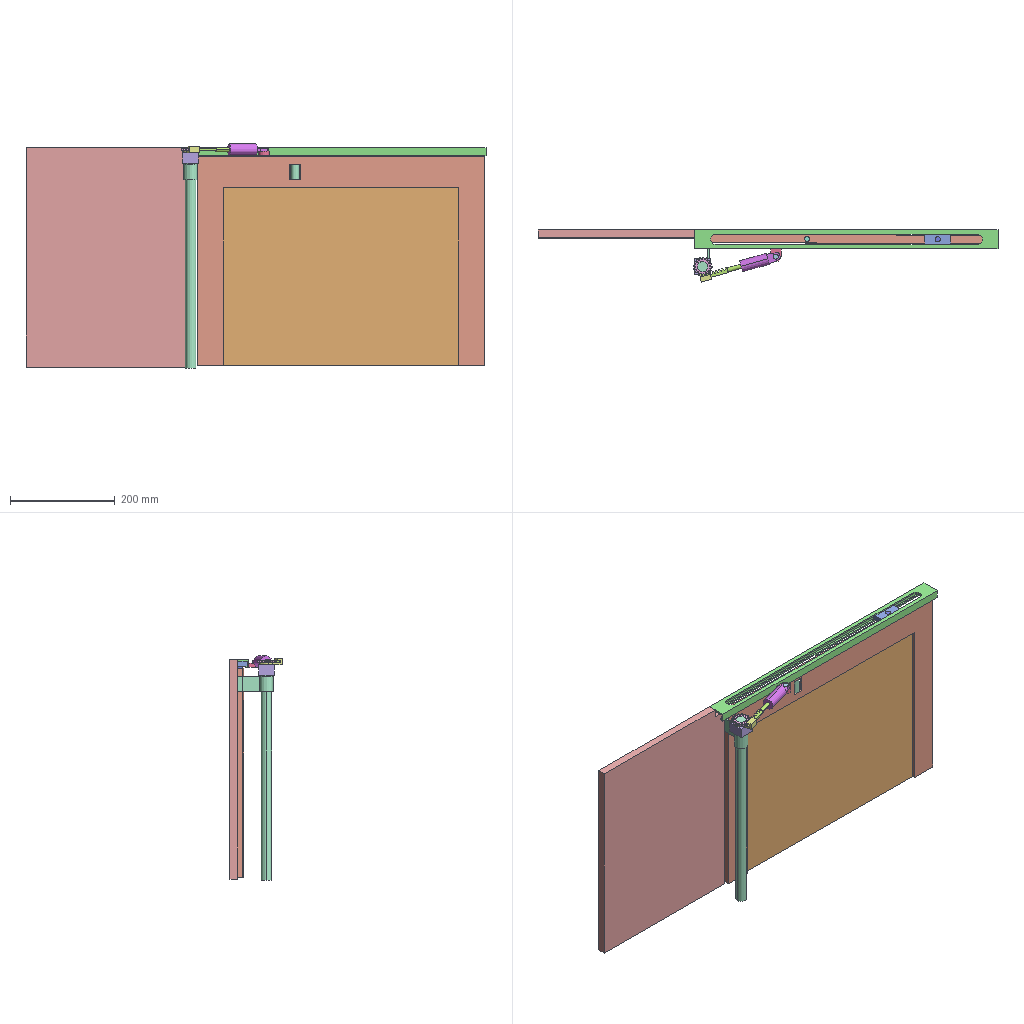Assembly | SolidWorks | 14 different items | 14 placed | box 880 x 100 x 429 mm
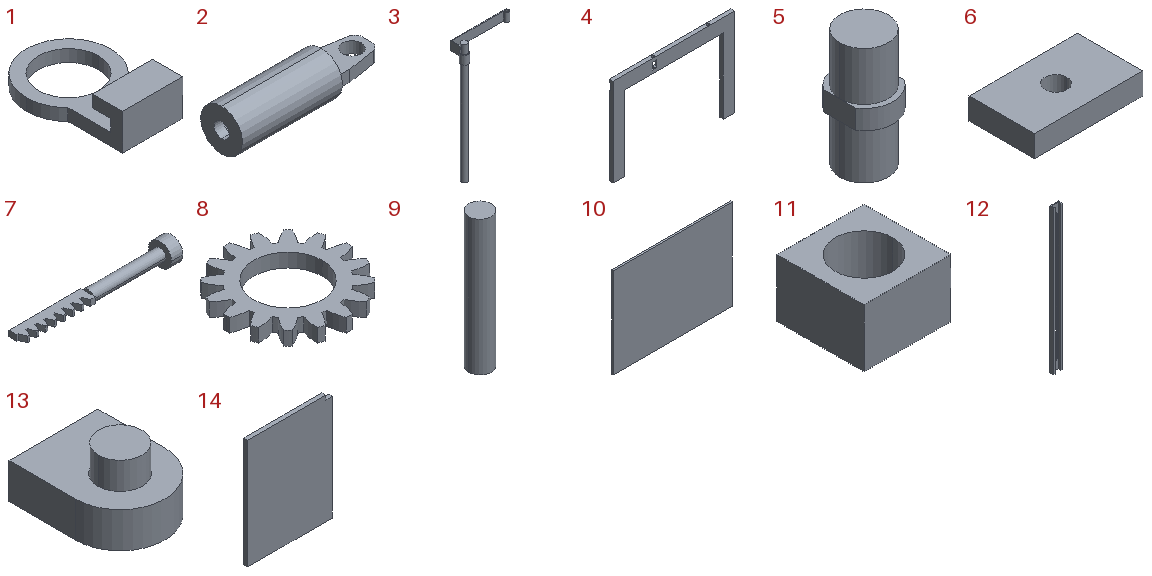Parts list (item | quantity | size | volume | features):
1 | x1 | 28 x 42 x 12 mm | 3551 mm3 | features ICE 2, Extrusion 1, HoleWzd 1
2 | x1 | 77 x 22 x 22 mm | 12617 mm3 | features HoleWzd 2, Fillet 1, ICE 1, Revolution 1
3 | x1 | 221 x 73 x 420 mm | 162659 mm3 | features ICE 2, Revolution 1
4 | x1 | 550 x 16 x 400 mm | 983083 mm3 | features ICE 10, HoleWzd 3, Extrusion 1
5 | x1 | 10 x 12 x 24 mm | 1987 mm3 | features Revolution 2, Extrusion 1
6 | x1 | 50 x 30 x 10 mm | 14215 mm3 | features Extrusion 1
7 | x1 | 108 x 16 x 16 mm | 5714 mm3 | features ICE 8, Extrusion 1, Revolution 1
8 | x1 | 36 x 36 x 4 mm | 1937 mm3 | features Extrusion 1
9 | x1 | 10 x 10 x 60 mm | 4712 mm3 | features Revolution 1
10 | x1 | 450 x 6 x 340 mm | 918000 mm3 | features Extrusion 1
11 | x1 | 30 x 30 x 20 mm | 11717 mm3 | features Extrusion 1
12 | x1 | 36 x 16 x 580 mm | 87378 mm3 | features ICE 2, Extrusion 1
13 | x1 | 20 x 25 x 14 mm | 4084 mm3 | features Extrusion 1, Revolution 1
14 | x1 | 325 x 15 x 420 mm | 2041500 mm3 | features Extrusion 1
Mates (type | each side: item.copy, entity, surface, feature):
Concentric | 3.1 face cylinder Boss-Extrude1 | 4.1 face cylinder Ø10.0 (10) Diameter Hole2
DistanceDim | 13.1 face plane Boss-Extrude1 | 12.1 face plane Boss-Extrude1 | 2 times
Coincident | 12.1 face plane Boss-Extrude1 | 13.1 face plane Boss-Extrude1
Coincident | 13.1 face plane Boss-Extrude1 | 2.1 face plane Boss-Extrude1
Concentric | 13.1 face cylinder Revolve2 | 2.1 face cylinder Ø10.0 (10) Diameter Hole1
Concentric | 7.1 face cylinder Revolve1 | 2.1 face cylinder Revolve1
Coincident | 6.1 face plane Boss-Extrude1 | 5.1 face plane Revolve1
Concentric | 6.1 face cylinder Boss-Extrude1 | 5.1 face cylinder Revolve1
DistanceDim | 11.1 face plane Boss-Extrude1 | 3.1 face plane Boss-Extrude1
Concentric | 1.1 face cylinder Ø20.0 (20) Diameter Hole1 | 3.1 face cylinder Revolve1
Concentric | 8.1 face cylinder Boss-Extrude1 | 3.1 face cylinder Revolve1
Coincident | 8.1 face plane Boss-Extrude1 | 1.1 face plane Boss-Extrude1
Parallel | 7.1 face plane Boss-Extrude1 | 1.1 face plane Boss-Extrude2
Parallel | 7.1 face plane Boss-Extrude1 | 1.1 face plane Boss-Extrude1
Coincident | 10.1 face plane Boss-Extrude1 | 4.1 face plane Boss-Extrude6
Width | 10.1 face plane Boss-Extrude1 | 10.1 face plane Boss-Extrude1 | 4.1 face plane Cut-Extrude5 | 4.1 face plane Cut-Extrude5
Concentric | 9.1 face cylinder Revolve1 | 4.1 face cylinder Ø10.0 (10) Diameter Hole2
Coincident | 9.1 face plane Revolve1 | 4.1 face plane Cut-Extrude5
Coincident | 14.1 face plane Boss-Extrude1 | 12.1 face plane Boss-Extrude1 | 2 times
Coincident | 7.1 face plane Boss-Extrude1 | 1.1 face plane Boss-Extrude2
Width | 6.1 face plane Boss-Extrude1 | 6.1 face plane Boss-Extrude1 | 12.1 face plane Cut-Extrude2 | 12.1 face plane Cut-Extrude2
Concentric | 11.1 face cylinder Boss-Extrude1 | 3.1 face cylinder Revolve1
Coincident | 3.1 face plane Boss-Extrude1 | 4.1 face plane Boss-Extrude6
Width | 10.1 face plane Boss-Extrude1 | 10.1 face plane Boss-Extrude1 | 4.1 face plane Boss-Extrude2 | 4.1 face plane Boss-Extrude3
Concentric | 4.1 face cylinder Ø10.0 (10) Diameter Hole1 | 5.1 face cylinder Revolve2
RackPinionDim | 7.1 select_type:24 | 8.1 select_type:24
Lock | 8.1 select_type:0 | 3.1 select_type:0
Coincident | 6.1 face plane Boss-Extrude1 | 12.1 face plane Cut-Extrude1
LimitDistanceDim | 7.1 face plane Boss-Extrude1 | 2.1 face plane Revolve1